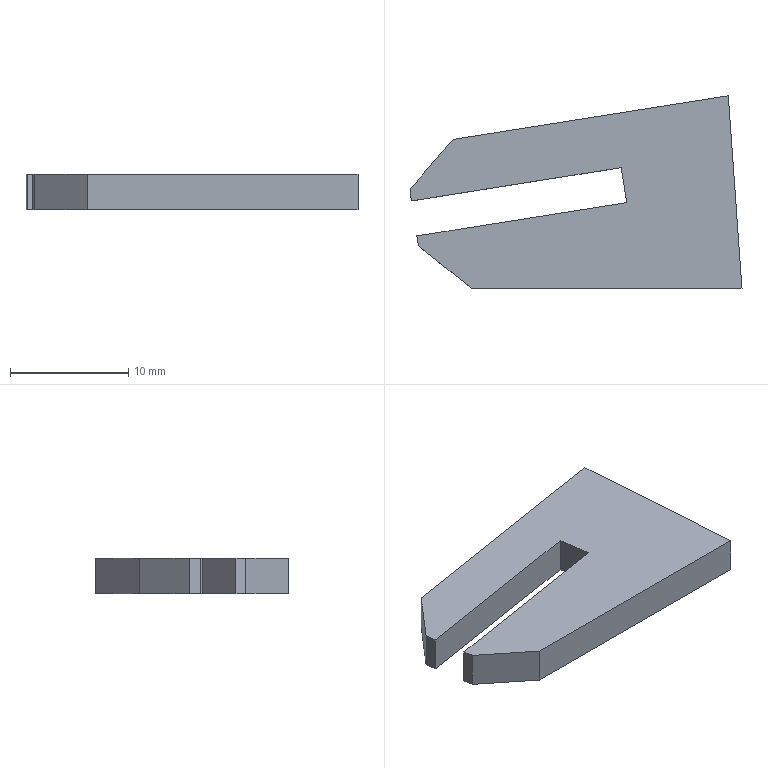Part | SolidWorks | features BaseBody 1 | 1 solid | 12 faces | box 28.09 x 16.288 x 3 mm | volume 953.359 mm3 | plane 12
STEP:
#1=CARTESIAN_POINT('',(-18.561,107.217,-1.5));
#2=VERTEX_POINT('',#1);
#3=CARTESIAN_POINT('',(-18.428,106.375,-1.5));
#4=VERTEX_POINT('',#3);
#5=CARTESIAN_POINT('',(-1.495,-0.2374,-1.5));
#6=DIRECTION('',(0.1569,-0.9876,0.));
#7=VECTOR('',#6,1000.);
#8=LINE('',#5,#7);
#9=EDGE_CURVE('',#2,#4,#8,.T.);
#10=ORIENTED_EDGE('',*,*,#9,.F.);
#11=CARTESIAN_POINT('',(-0.8058,110.036,-1.5));
#12=VERTEX_POINT('',#11);
#13=CARTESIAN_POINT('',(-17.06,107.455,-1.5));
#14=DIRECTION('',(0.9876,0.1568,0.));
#15=VECTOR('',#14,1000.);
#16=LINE('',#13,#15);
#17=EDGE_CURVE('',#2,#12,#16,.T.);
#18=ORIENTED_EDGE('',*,*,#17,.T.);
#19=CARTESIAN_POINT('',(-1.276,112.999,-1.5));
#20=VERTEX_POINT('',#19);
#21=CARTESIAN_POINT('',(16.255,2.581,-1.5));
#22=DIRECTION('',(-0.1568,0.9876,0.));
#23=VECTOR('',#22,1000.);
#24=LINE('',#21,#23);
#25=EDGE_CURVE('',#12,#20,#24,.T.);
#26=ORIENTED_EDGE('',*,*,#25,.T.);
#27=CARTESIAN_POINT('',(-19.031,110.18,-1.5));
#28=VERTEX_POINT('',#27);
#29=CARTESIAN_POINT('',(-17.531,110.418,-1.5));
#30=DIRECTION('',(0.9876,0.1568,0.));
#31=VECTOR('',#30,1000.);
#32=LINE('',#29,#31);
#33=EDGE_CURVE('',#28,#20,#32,.T.);
#34=ORIENTED_EDGE('',*,*,#33,.F.);
#35=CARTESIAN_POINT('',(-19.143,111.169,-1.5));
#36=VERTEX_POINT('',#35);
#37=CARTESIAN_POINT('',(-6.473,-0.7329,-1.5));
#38=DIRECTION('',(-0.1125,0.9937,0.));
#39=VECTOR('',#38,1000.);
#40=LINE('',#37,#39);
#41=EDGE_CURVE('',#28,#36,#40,.T.);
#42=ORIENTED_EDGE('',*,*,#41,.T.);
#43=CARTESIAN_POINT('',(-15.505,115.389,-1.5));
#44=VERTEX_POINT('',#43);
#45=CARTESIAN_POINT('',(-65.96,56.859,-1.5));
#46=DIRECTION('',(-0.6529,-0.7574,0.));
#47=VECTOR('',#46,1000.);
#48=LINE('',#45,#47);
#49=EDGE_CURVE('',#44,#36,#48,.T.);
#50=ORIENTED_EDGE('',*,*,#49,.F.);
#51=CARTESIAN_POINT('',(7.784,119.082,-1.5));
#52=VERTEX_POINT('',#51);
#53=CARTESIAN_POINT('',(-18.226,114.958,-1.5));
#54=DIRECTION('',(0.9877,0.1566,0.));
#55=VECTOR('',#54,1000.);
#56=LINE('',#53,#55);
#57=EDGE_CURVE('',#44,#52,#56,.T.);
#58=ORIENTED_EDGE('',*,*,#57,.T.);
#59=CARTESIAN_POINT('',(8.947,102.795,-1.5));
#60=VERTEX_POINT('',#59);
#61=CARTESIAN_POINT('',(16.204,1.157,-1.5));
#62=DIRECTION('',(0.07122,-0.9975,0.));
#63=VECTOR('',#62,1000.);
#64=LINE('',#61,#63);
#65=EDGE_CURVE('',#52,#60,#64,.T.);
#66=ORIENTED_EDGE('',*,*,#65,.T.);
#67=CARTESIAN_POINT('',(-13.951,102.794,-1.5));
#68=VERTEX_POINT('',#67);
#69=CARTESIAN_POINT('',(-0.006828,102.795,-1.5));
#70=DIRECTION('',(1.,0.00006642,0.));
#71=VECTOR('',#70,1000.);
#72=LINE('',#69,#71);
#73=EDGE_CURVE('',#68,#60,#72,.T.);
#74=ORIENTED_EDGE('',*,*,#73,.F.);
#75=CARTESIAN_POINT('',(44.699,55.878,-1.5));
#76=DIRECTION('',(0.7809,-0.6247,0.));
#77=VECTOR('',#76,1000.);
#78=LINE('',#75,#77);
#79=EDGE_CURVE('',#4,#68,#78,.T.);
#80=ORIENTED_EDGE('',*,*,#79,.F.);
#81=EDGE_LOOP('',(#10,#18,#26,#34,#42,#50,#58,#66,#74,#80));
#82=FACE_OUTER_BOUND('',#81,.T.);
#83=CARTESIAN_POINT('',(0.,0.,-1.5));
#84=DIRECTION('',(0.,0.,1.));
#85=DIRECTION('',(1.,0.,0.));
#86=AXIS2_PLACEMENT_3D('',#83,#84,#85);
#87=PLANE('',#86);
#88=ADVANCED_FACE('',(#82),#87,.F.);
#89=CARTESIAN_POINT('',(-18.561,107.217,1.5));
#90=VERTEX_POINT('',#89);
#91=CARTESIAN_POINT('',(-18.428,106.375,1.5));
#92=VERTEX_POINT('',#91);
#93=CARTESIAN_POINT('',(-1.495,-0.2374,1.5));
#94=DIRECTION('',(0.1569,-0.9876,0.));
#95=VECTOR('',#94,1000.);
#96=LINE('',#93,#95);
#97=EDGE_CURVE('',#90,#92,#96,.T.);
#98=ORIENTED_EDGE('',*,*,#97,.T.);
#99=CARTESIAN_POINT('',(-13.951,102.794,1.5));
#100=VERTEX_POINT('',#99);
#101=CARTESIAN_POINT('',(44.699,55.878,1.5));
#102=DIRECTION('',(0.7809,-0.6247,0.));
#103=VECTOR('',#102,1000.);
#104=LINE('',#101,#103);
#105=EDGE_CURVE('',#92,#100,#104,.T.);
#106=ORIENTED_EDGE('',*,*,#105,.T.);
#107=CARTESIAN_POINT('',(8.947,102.795,1.5));
#108=VERTEX_POINT('',#107);
#109=CARTESIAN_POINT('',(-0.006828,102.795,1.5));
#110=DIRECTION('',(1.,0.00006642,0.));
#111=VECTOR('',#110,1000.);
#112=LINE('',#109,#111);
#113=EDGE_CURVE('',#100,#108,#112,.T.);
#114=ORIENTED_EDGE('',*,*,#113,.T.);
#115=CARTESIAN_POINT('',(7.784,119.082,1.5));
#116=VERTEX_POINT('',#115);
#117=CARTESIAN_POINT('',(16.204,1.157,1.5));
#118=DIRECTION('',(0.07122,-0.9975,0.));
#119=VECTOR('',#118,1000.);
#120=LINE('',#117,#119);
#121=EDGE_CURVE('',#116,#108,#120,.T.);
#122=ORIENTED_EDGE('',*,*,#121,.F.);
#123=CARTESIAN_POINT('',(-15.505,115.389,1.5));
#124=VERTEX_POINT('',#123);
#125=CARTESIAN_POINT('',(-18.226,114.958,1.5));
#126=DIRECTION('',(0.9877,0.1566,0.));
#127=VECTOR('',#126,1000.);
#128=LINE('',#125,#127);
#129=EDGE_CURVE('',#124,#116,#128,.T.);
#130=ORIENTED_EDGE('',*,*,#129,.F.);
#131=CARTESIAN_POINT('',(-19.143,111.169,1.5));
#132=VERTEX_POINT('',#131);
#133=CARTESIAN_POINT('',(-65.96,56.859,1.5));
#134=DIRECTION('',(-0.6529,-0.7574,0.));
#135=VECTOR('',#134,1000.);
#136=LINE('',#133,#135);
#137=EDGE_CURVE('',#124,#132,#136,.T.);
#138=ORIENTED_EDGE('',*,*,#137,.T.);
#139=CARTESIAN_POINT('',(-19.031,110.18,1.5));
#140=VERTEX_POINT('',#139);
#141=CARTESIAN_POINT('',(-6.473,-0.7329,1.5));
#142=DIRECTION('',(-0.1125,0.9937,0.));
#143=VECTOR('',#142,1000.);
#144=LINE('',#141,#143);
#145=EDGE_CURVE('',#140,#132,#144,.T.);
#146=ORIENTED_EDGE('',*,*,#145,.F.);
#147=CARTESIAN_POINT('',(-1.276,112.999,1.5));
#148=VERTEX_POINT('',#147);
#149=CARTESIAN_POINT('',(-17.531,110.418,1.5));
#150=DIRECTION('',(0.9876,0.1568,0.));
#151=VECTOR('',#150,1000.);
#152=LINE('',#149,#151);
#153=EDGE_CURVE('',#140,#148,#152,.T.);
#154=ORIENTED_EDGE('',*,*,#153,.T.);
#155=CARTESIAN_POINT('',(-0.8058,110.036,1.5));
#156=VERTEX_POINT('',#155);
#157=CARTESIAN_POINT('',(16.255,2.581,1.5));
#158=DIRECTION('',(-0.1568,0.9876,0.));
#159=VECTOR('',#158,1000.);
#160=LINE('',#157,#159);
#161=EDGE_CURVE('',#156,#148,#160,.T.);
#162=ORIENTED_EDGE('',*,*,#161,.F.);
#163=CARTESIAN_POINT('',(-17.06,107.455,1.5));
#164=DIRECTION('',(0.9876,0.1568,0.));
#165=VECTOR('',#164,1000.);
#166=LINE('',#163,#165);
#167=EDGE_CURVE('',#90,#156,#166,.T.);
#168=ORIENTED_EDGE('',*,*,#167,.F.);
#169=EDGE_LOOP('',(#98,#106,#114,#122,#130,#138,#146,#154,#162,#168));
#170=FACE_OUTER_BOUND('',#169,.T.);
#171=CARTESIAN_POINT('',(0.,0.,1.5));
#172=DIRECTION('',(0.,0.,1.));
#173=DIRECTION('',(1.,0.,0.));
#174=AXIS2_PLACEMENT_3D('',#171,#172,#173);
#175=PLANE('',#174);
#176=ADVANCED_FACE('',(#170),#175,.T.);
#177=ORIENTED_EDGE('',*,*,#17,.F.);
#178=CARTESIAN_POINT('',(-18.561,107.217,1.5));
#179=DIRECTION('',(0.,0.,-1.));
#180=VECTOR('',#179,1000.);
#181=LINE('',#178,#180);
#182=EDGE_CURVE('',#90,#2,#181,.T.);
#183=ORIENTED_EDGE('',*,*,#182,.F.);
#184=ORIENTED_EDGE('',*,*,#167,.T.);
#185=CARTESIAN_POINT('',(-0.8058,110.036,1.5));
#186=DIRECTION('',(0.,0.,-1.));
#187=VECTOR('',#186,1000.);
#188=LINE('',#185,#187);
#189=EDGE_CURVE('',#156,#12,#188,.T.);
#190=ORIENTED_EDGE('',*,*,#189,.T.);
#191=EDGE_LOOP('',(#177,#183,#184,#190));
#192=FACE_OUTER_BOUND('',#191,.T.);
#193=CARTESIAN_POINT('',(-17.06,107.455,1.5));
#194=DIRECTION('',(-0.1568,0.9876,0.));
#195=DIRECTION('',(0.,0.,1.));
#196=AXIS2_PLACEMENT_3D('',#193,#194,#195);
#197=PLANE('',#196);
#198=ADVANCED_FACE('',(#192),#197,.T.);
#199=ORIENTED_EDGE('',*,*,#25,.F.);
#200=ORIENTED_EDGE('',*,*,#189,.F.);
#201=ORIENTED_EDGE('',*,*,#161,.T.);
#202=CARTESIAN_POINT('',(-1.276,112.999,1.5));
#203=DIRECTION('',(0.,0.,-1.));
#204=VECTOR('',#203,1000.);
#205=LINE('',#202,#204);
#206=EDGE_CURVE('',#148,#20,#205,.T.);
#207=ORIENTED_EDGE('',*,*,#206,.T.);
#208=EDGE_LOOP('',(#199,#200,#201,#207));
#209=FACE_OUTER_BOUND('',#208,.T.);
#210=CARTESIAN_POINT('',(16.255,2.581,1.5));
#211=DIRECTION('',(-0.9876,-0.1568,0.));
#212=DIRECTION('',(-0.1568,0.9876,0.));
#213=AXIS2_PLACEMENT_3D('',#210,#211,#212);
#214=PLANE('',#213);
#215=ADVANCED_FACE('',(#209),#214,.T.);
#216=ORIENTED_EDGE('',*,*,#33,.T.);
#217=ORIENTED_EDGE('',*,*,#206,.F.);
#218=ORIENTED_EDGE('',*,*,#153,.F.);
#219=CARTESIAN_POINT('',(-19.031,110.18,1.5));
#220=DIRECTION('',(0.,0.,-1.));
#221=VECTOR('',#220,1000.);
#222=LINE('',#219,#221);
#223=EDGE_CURVE('',#140,#28,#222,.T.);
#224=ORIENTED_EDGE('',*,*,#223,.T.);
#225=EDGE_LOOP('',(#216,#217,#218,#224));
#226=FACE_OUTER_BOUND('',#225,.T.);
#227=CARTESIAN_POINT('',(-17.531,110.418,1.5));
#228=DIRECTION('',(-0.1568,0.9876,0.));
#229=DIRECTION('',(0.,0.,1.));
#230=AXIS2_PLACEMENT_3D('',#227,#228,#229);
#231=PLANE('',#230);
#232=ADVANCED_FACE('',(#226),#231,.F.);
#233=ORIENTED_EDGE('',*,*,#41,.F.);
#234=ORIENTED_EDGE('',*,*,#223,.F.);
#235=ORIENTED_EDGE('',*,*,#145,.T.);
#236=CARTESIAN_POINT('',(-19.143,111.169,1.5));
#237=DIRECTION('',(0.,0.,-1.));
#238=VECTOR('',#237,1000.);
#239=LINE('',#236,#238);
#240=EDGE_CURVE('',#132,#36,#239,.T.);
#241=ORIENTED_EDGE('',*,*,#240,.T.);
#242=EDGE_LOOP('',(#233,#234,#235,#241));
#243=FACE_OUTER_BOUND('',#242,.T.);
#244=CARTESIAN_POINT('',(-6.473,-0.7329,1.5));
#245=DIRECTION('',(-0.9937,-0.1125,0.));
#246=DIRECTION('',(-0.1125,0.9937,0.));
#247=AXIS2_PLACEMENT_3D('',#244,#245,#246);
#248=PLANE('',#247);
#249=ADVANCED_FACE('',(#243),#248,.T.);
#250=ORIENTED_EDGE('',*,*,#49,.T.);
#251=ORIENTED_EDGE('',*,*,#240,.F.);
#252=ORIENTED_EDGE('',*,*,#137,.F.);
#253=CARTESIAN_POINT('',(-15.505,115.389,1.5));
#254=DIRECTION('',(0.,0.,-1.));
#255=VECTOR('',#254,1000.);
#256=LINE('',#253,#255);
#257=EDGE_CURVE('',#124,#44,#256,.T.);
#258=ORIENTED_EDGE('',*,*,#257,.T.);
#259=EDGE_LOOP('',(#250,#251,#252,#258));
#260=FACE_OUTER_BOUND('',#259,.T.);
#261=CARTESIAN_POINT('',(-65.96,56.859,1.5));
#262=DIRECTION('',(0.7574,-0.6529,0.));
#263=DIRECTION('',(0.,0.,-1.));
#264=AXIS2_PLACEMENT_3D('',#261,#262,#263);
#265=PLANE('',#264);
#266=ADVANCED_FACE('',(#260),#265,.F.);
#267=ORIENTED_EDGE('',*,*,#57,.F.);
#268=ORIENTED_EDGE('',*,*,#257,.F.);
#269=ORIENTED_EDGE('',*,*,#129,.T.);
#270=CARTESIAN_POINT('',(7.784,119.082,1.5));
#271=DIRECTION('',(0.,0.,-1.));
#272=VECTOR('',#271,1000.);
#273=LINE('',#270,#272);
#274=EDGE_CURVE('',#116,#52,#273,.T.);
#275=ORIENTED_EDGE('',*,*,#274,.T.);
#276=EDGE_LOOP('',(#267,#268,#269,#275));
#277=FACE_OUTER_BOUND('',#276,.T.);
#278=CARTESIAN_POINT('',(-18.226,114.958,1.5));
#279=DIRECTION('',(-0.1566,0.9877,0.));
#280=DIRECTION('',(0.,0.,1.));
#281=AXIS2_PLACEMENT_3D('',#278,#279,#280);
#282=PLANE('',#281);
#283=ADVANCED_FACE('',(#277),#282,.T.);
#284=ORIENTED_EDGE('',*,*,#65,.F.);
#285=ORIENTED_EDGE('',*,*,#274,.F.);
#286=ORIENTED_EDGE('',*,*,#121,.T.);
#287=CARTESIAN_POINT('',(8.947,102.795,1.5));
#288=DIRECTION('',(0.,0.,-1.));
#289=VECTOR('',#288,1000.);
#290=LINE('',#287,#289);
#291=EDGE_CURVE('',#108,#60,#290,.T.);
#292=ORIENTED_EDGE('',*,*,#291,.T.);
#293=EDGE_LOOP('',(#284,#285,#286,#292));
#294=FACE_OUTER_BOUND('',#293,.T.);
#295=CARTESIAN_POINT('',(16.204,1.157,1.5));
#296=DIRECTION('',(0.9975,0.07122,0.));
#297=DIRECTION('',(0.,0.,-1.));
#298=AXIS2_PLACEMENT_3D('',#295,#296,#297);
#299=PLANE('',#298);
#300=ADVANCED_FACE('',(#294),#299,.T.);
#301=ORIENTED_EDGE('',*,*,#73,.T.);
#302=ORIENTED_EDGE('',*,*,#291,.F.);
#303=ORIENTED_EDGE('',*,*,#113,.F.);
#304=CARTESIAN_POINT('',(-13.951,102.794,1.5));
#305=DIRECTION('',(0.,0.,-1.));
#306=VECTOR('',#305,1000.);
#307=LINE('',#304,#306);
#308=EDGE_CURVE('',#100,#68,#307,.T.);
#309=ORIENTED_EDGE('',*,*,#308,.T.);
#310=EDGE_LOOP('',(#301,#302,#303,#309));
#311=FACE_OUTER_BOUND('',#310,.T.);
#312=CARTESIAN_POINT('',(-0.006828,102.795,1.5));
#313=DIRECTION('',(-0.00006642,1.,0.));
#314=DIRECTION('',(0.,0.,1.));
#315=AXIS2_PLACEMENT_3D('',#312,#313,#314);
#316=PLANE('',#315);
#317=ADVANCED_FACE('',(#311),#316,.F.);
#318=ORIENTED_EDGE('',*,*,#79,.T.);
#319=ORIENTED_EDGE('',*,*,#308,.F.);
#320=ORIENTED_EDGE('',*,*,#105,.F.);
#321=CARTESIAN_POINT('',(-18.428,106.375,1.5));
#322=DIRECTION('',(0.,0.,-1.));
#323=VECTOR('',#322,1000.);
#324=LINE('',#321,#323);
#325=EDGE_CURVE('',#92,#4,#324,.T.);
#326=ORIENTED_EDGE('',*,*,#325,.T.);
#327=EDGE_LOOP('',(#318,#319,#320,#326));
#328=FACE_OUTER_BOUND('',#327,.T.);
#329=CARTESIAN_POINT('',(44.699,55.878,1.5));
#330=DIRECTION('',(0.6247,0.7809,0.));
#331=DIRECTION('',(0.,0.,-1.));
#332=AXIS2_PLACEMENT_3D('',#329,#330,#331);
#333=PLANE('',#332);
#334=ADVANCED_FACE('',(#328),#333,.F.);
#335=ORIENTED_EDGE('',*,*,#9,.T.);
#336=ORIENTED_EDGE('',*,*,#325,.F.);
#337=ORIENTED_EDGE('',*,*,#97,.F.);
#338=ORIENTED_EDGE('',*,*,#182,.T.);
#339=EDGE_LOOP('',(#335,#336,#337,#338));
#340=FACE_OUTER_BOUND('',#339,.T.);
#341=CARTESIAN_POINT('',(-1.495,-0.2374,1.5));
#342=DIRECTION('',(0.9876,0.1569,0.));
#343=DIRECTION('',(0.,0.,-1.));
#344=AXIS2_PLACEMENT_3D('',#341,#342,#343);
#345=PLANE('',#344);
#346=ADVANCED_FACE('',(#340),#345,.F.);
#347=CLOSED_SHELL('',(#88,#176,#198,#215,#232,#249,#266,#283,#300,#317,#334,#346));
#348=MANIFOLD_SOLID_BREP('',#347);
#349=CARTESIAN_POINT('',(0.,0.,0.));
#350=DIRECTION('',(0.,0.,1.));
#351=DIRECTION('',(1.,0.,0.));
#352=AXIS2_PLACEMENT_3D('',#349,#350,#351);
#353=(LENGTH_UNIT()NAMED_UNIT(*)SI_UNIT(.MILLI.,.METRE.));
#354=UNCERTAINTY_MEASURE_WITH_UNIT(LENGTH_MEASURE(0.00001),#353,'','');
#355=(NAMED_UNIT(*)PLANE_ANGLE_UNIT()SI_UNIT($,.RADIAN.));
#356=(NAMED_UNIT(*)SI_UNIT($,.STERADIAN.)SOLID_ANGLE_UNIT());
#357=(GEOMETRIC_REPRESENTATION_CONTEXT(3)GLOBAL_UNCERTAINTY_ASSIGNED_CONTEXT((#354))GLOBAL_UNIT_ASSIGNED_CONTEXT((#353,#355,#356))REPRESENTATION_CONTEXT('',''));
#358=ADVANCED_BREP_SHAPE_REPRESENTATION('',(#348,#352),#357);